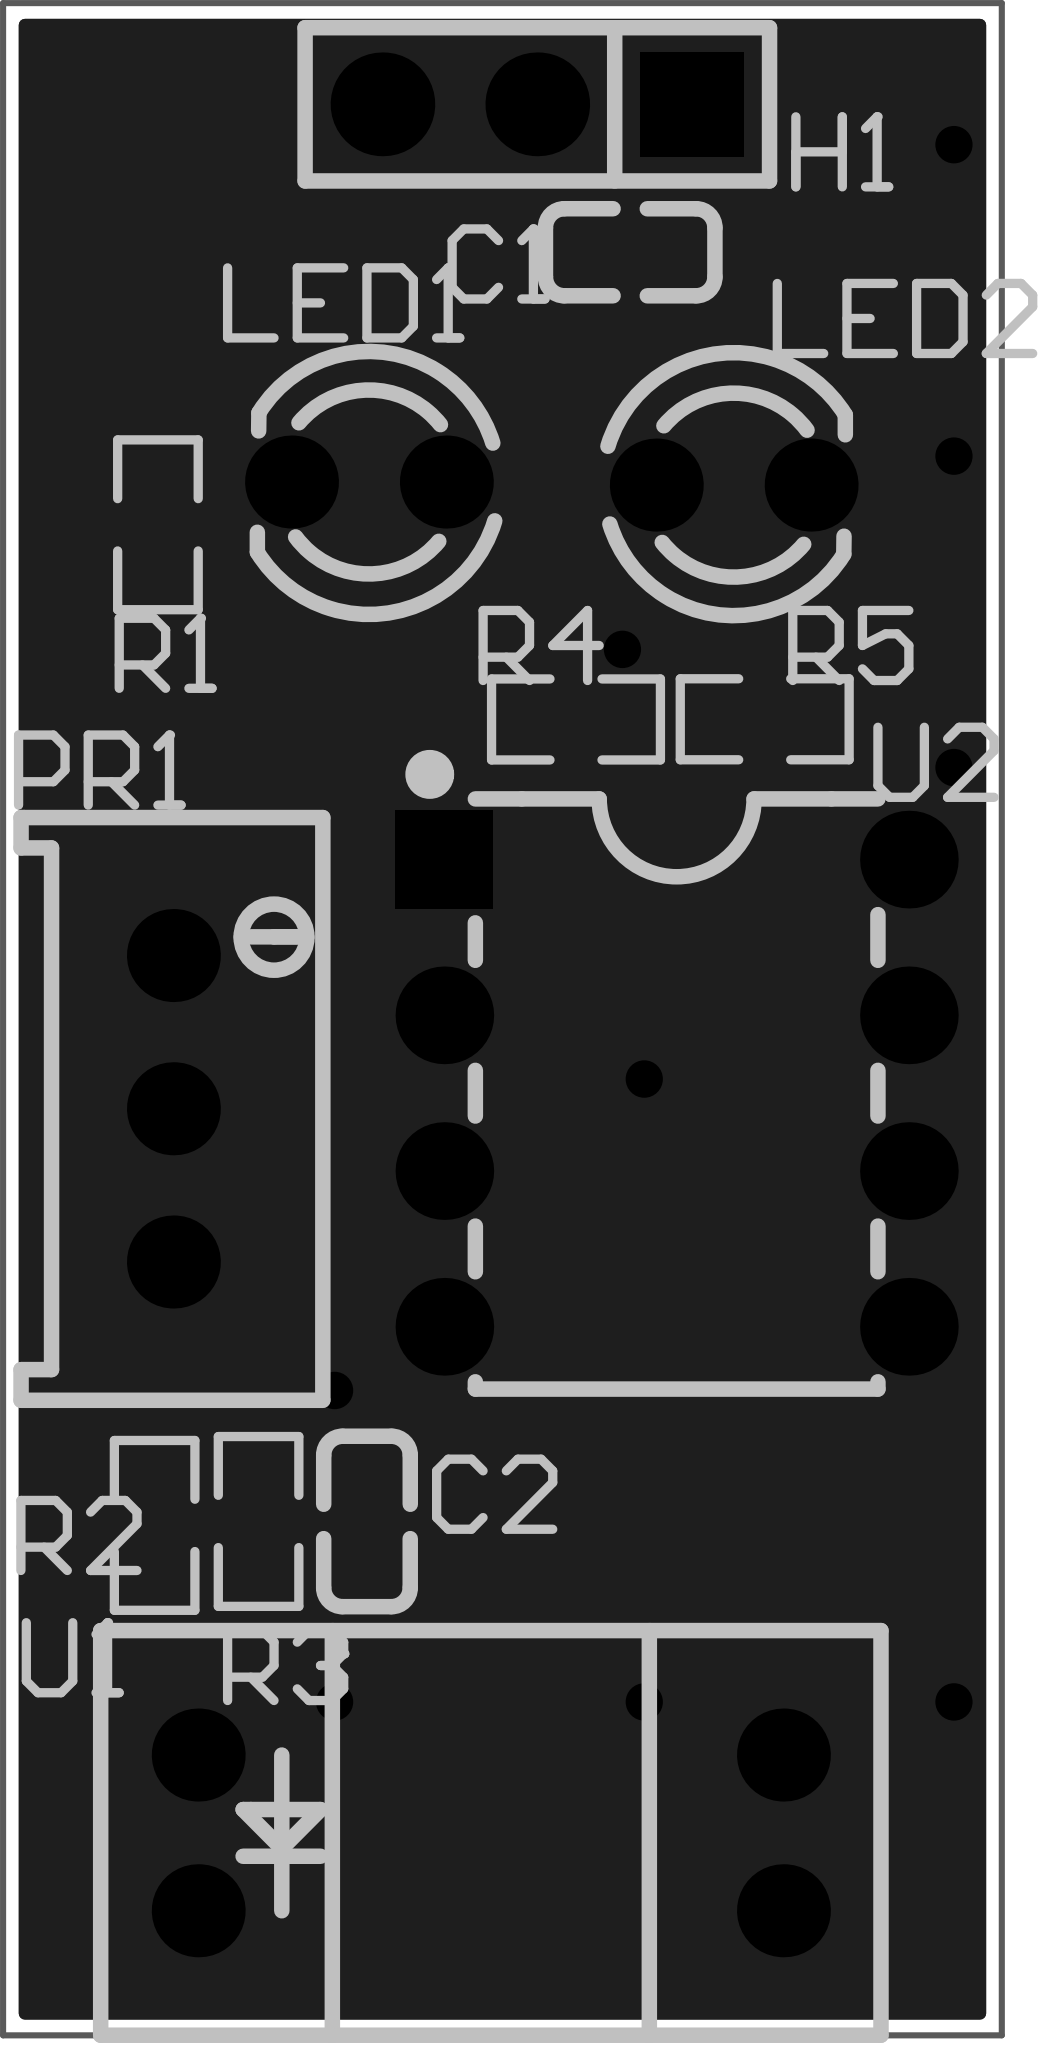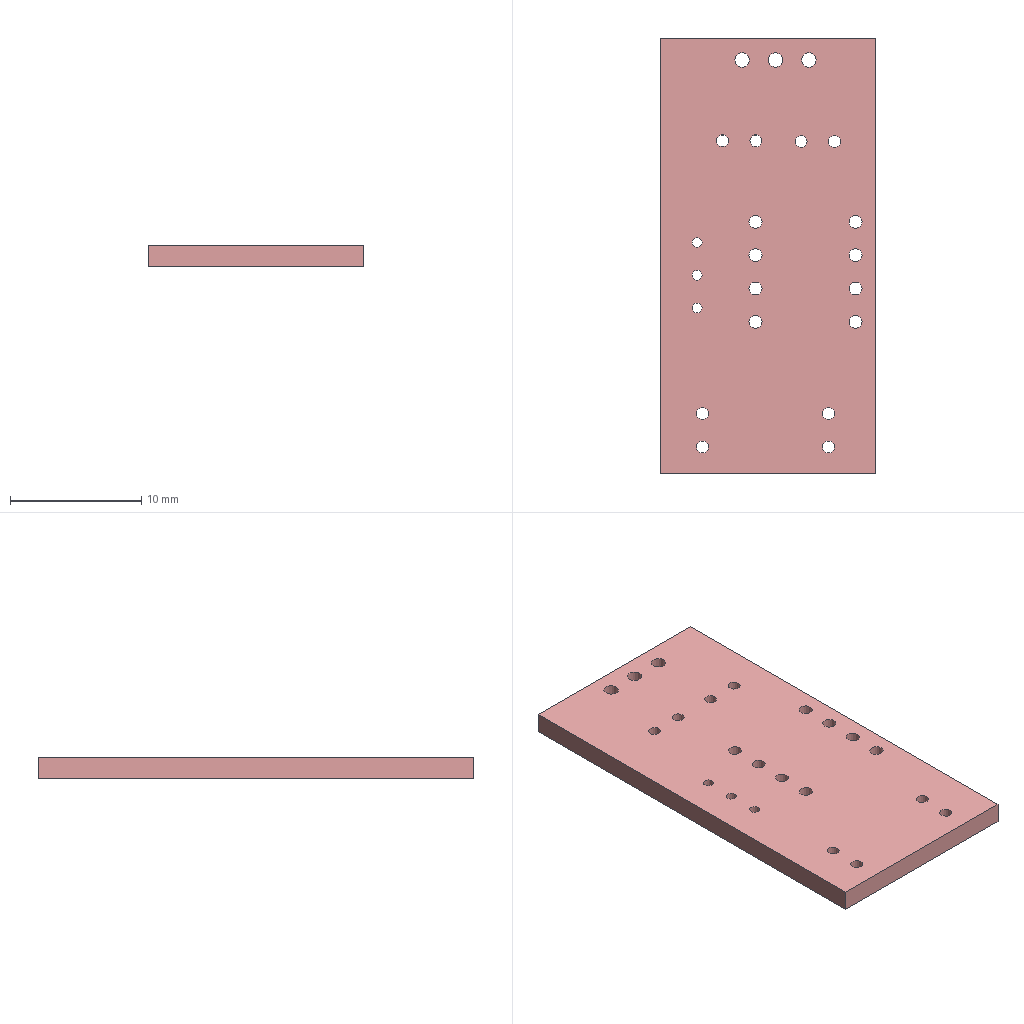Circuit board layout | Altium Designer | box 16.4 x 33.1 x 1.6 mm
Layer stack:
# Altium Designer layer stack of  (unit mm; dielectric type: 0 none, 1 core, 2 prepreg, 3 surface material)
index,name,kind,layer,copper_thickness_mm,dielectric_type,dielectric_thickness_mm,dielectric_material,dielectric_constant
0,Top Paste Mask Layer,other,,,,,,
1,Top Silkscreen Layer,other,,,,,,
2,Top Solder Mask Layer,dielectric,,,3,0.01,,3.3
3,Top Layer,copper,Top Layer,0.035,,,,
4,Dielectric1,dielectric,,,3,1.51,FR4,4.5
5,Bottom Layer,copper,Bottom Layer,0.035,,,,
6,Bottom Solder Mask Layer,dielectric,,,3,0.01,,3.3
7,Bottom Silkscreen Layer,other,,,,,,
8,Bottom Paste Mask Layer,other,,,,,,
# drill layer pairs: low layer,high layer
drill_pair,Top Layer,Bottom Layer
Part placement:
Designator,Comment,Layer,Footprint,Center-X(mm),Center-Y(mm),Rotation
C1,100nF,TopLayer,C0603,91.44,109.347,0
C2,100nF,TopLayer,C0603,87.122,88.646,270
H1,,TopLayer,HDR-TH_3P-P2.54-V-M,89.916,111.76,180
LED1,,TopLayer,LED_TH-3mm,87.154,105.6,180
LED2,,TopLayer,LED_TH-3mm,93.139,105.55,0
PR1,10kΩ,TopLayer,R_3296,83.947,95.377,270
R1,1K,TopLayer,R0603,83.693,104.902,90
R2,100,TopLayer,R0603,83.639,88.582,90
R3,10K,TopLayer,R0603,85.344,88.646,90
R4,10K,TopLayer,R0603,90.551,101.727,180
R5,1K,TopLayer,R0603,93.647,101.73,0
U1,ZOS-T1305-A02(ZD),TopLayer,OPTO-TH_ZOS-T1305-A02,89.154,83.566,0
U2,LM393N-ON,TopLayer,PDIP-8_L9.6-W6.4-P2.54-LS7.9-BL,92.202,95.631,270
Pad and via stacks:
# Altium Designer via and pad stacks of  (unit mm). Each distinct definition once, with the count of objects using it.
# via: kind,start_layer,end_layer,hole_mm,diameter_mm,mode(0 simple;1 top-mid-bottom;2 full stack),diameter_per_layer,count,example_net
# pad: kind,layer,hole_mm,hole_type(0 round;1 square;2 slot),plating,top_size,top_shape(1 round;2 rect;3 octagon;9 rounded rect),mid_size,bottom_size,mode,footprint,size_per_layer,count,example
pad,Top Layer,0,0,plated,0.8x0.9,2,0.8x0.9,0.8x0.9,0,C0603,,4,C1.2
pad,Top Layer,0,0,plated,0.8065x0.864,2,0.8065x0.864,0.8065x0.864,0,R0603,,10,R1.2
pad,Multi-Layer,1.1,0,plated,1.7x1.7,2,1.7x1.7,1.7x1.7,0,HDR-TH_3P-P2.54-V-M,,1,H1.1
pad,Multi-Layer,1.1,0,plated,1.7x1.7,1,1.7x1.7,1.7x1.7,0,HDR-TH_3P-P2.54-V-M,,2,H1.2
pad,Multi-Layer,0.9144,0,plated,1.524x1.524,1,1.524x1.524,1.524x1.524,0,LED_TH-3mm,,4,LED1.1
pad,Multi-Layer,0.762,0,plated,1.524x1.524,1,1.524x1.524,1.524x1.524,0,R_3296,,3,PR1.2
pad,Multi-Layer,0.9144,0,plated,1.524x1.524,1,1.524x1.524,1.524x1.524,0,OPTO-TH_ZOS-T1305-A02,,4,U1.1
pad,Multi-Layer,1,0,plated,1.6x1.6,2,1.6x1.6,1.6x1.6,0,PDIP-8_L9.6-W6.4-P2.54-LS7.9-BL,,1,U2.1
pad,Multi-Layer,1,0,plated,1.6x1.6,1,1.6x1.6,1.6x1.6,0,PDIP-8_L9.6-W6.4-P2.54-LS7.9-BL,,7,U2.2
via,Top Layer,Bottom Layer,0.3048,0.61,0,,9,DO
Copper pours:
name,layer,net,type(0 solid;1 hatched;2 none)
Top Layer-GND,Top Layer,GND,0
Bottom Layer-GND,Bottom Layer,GND,0